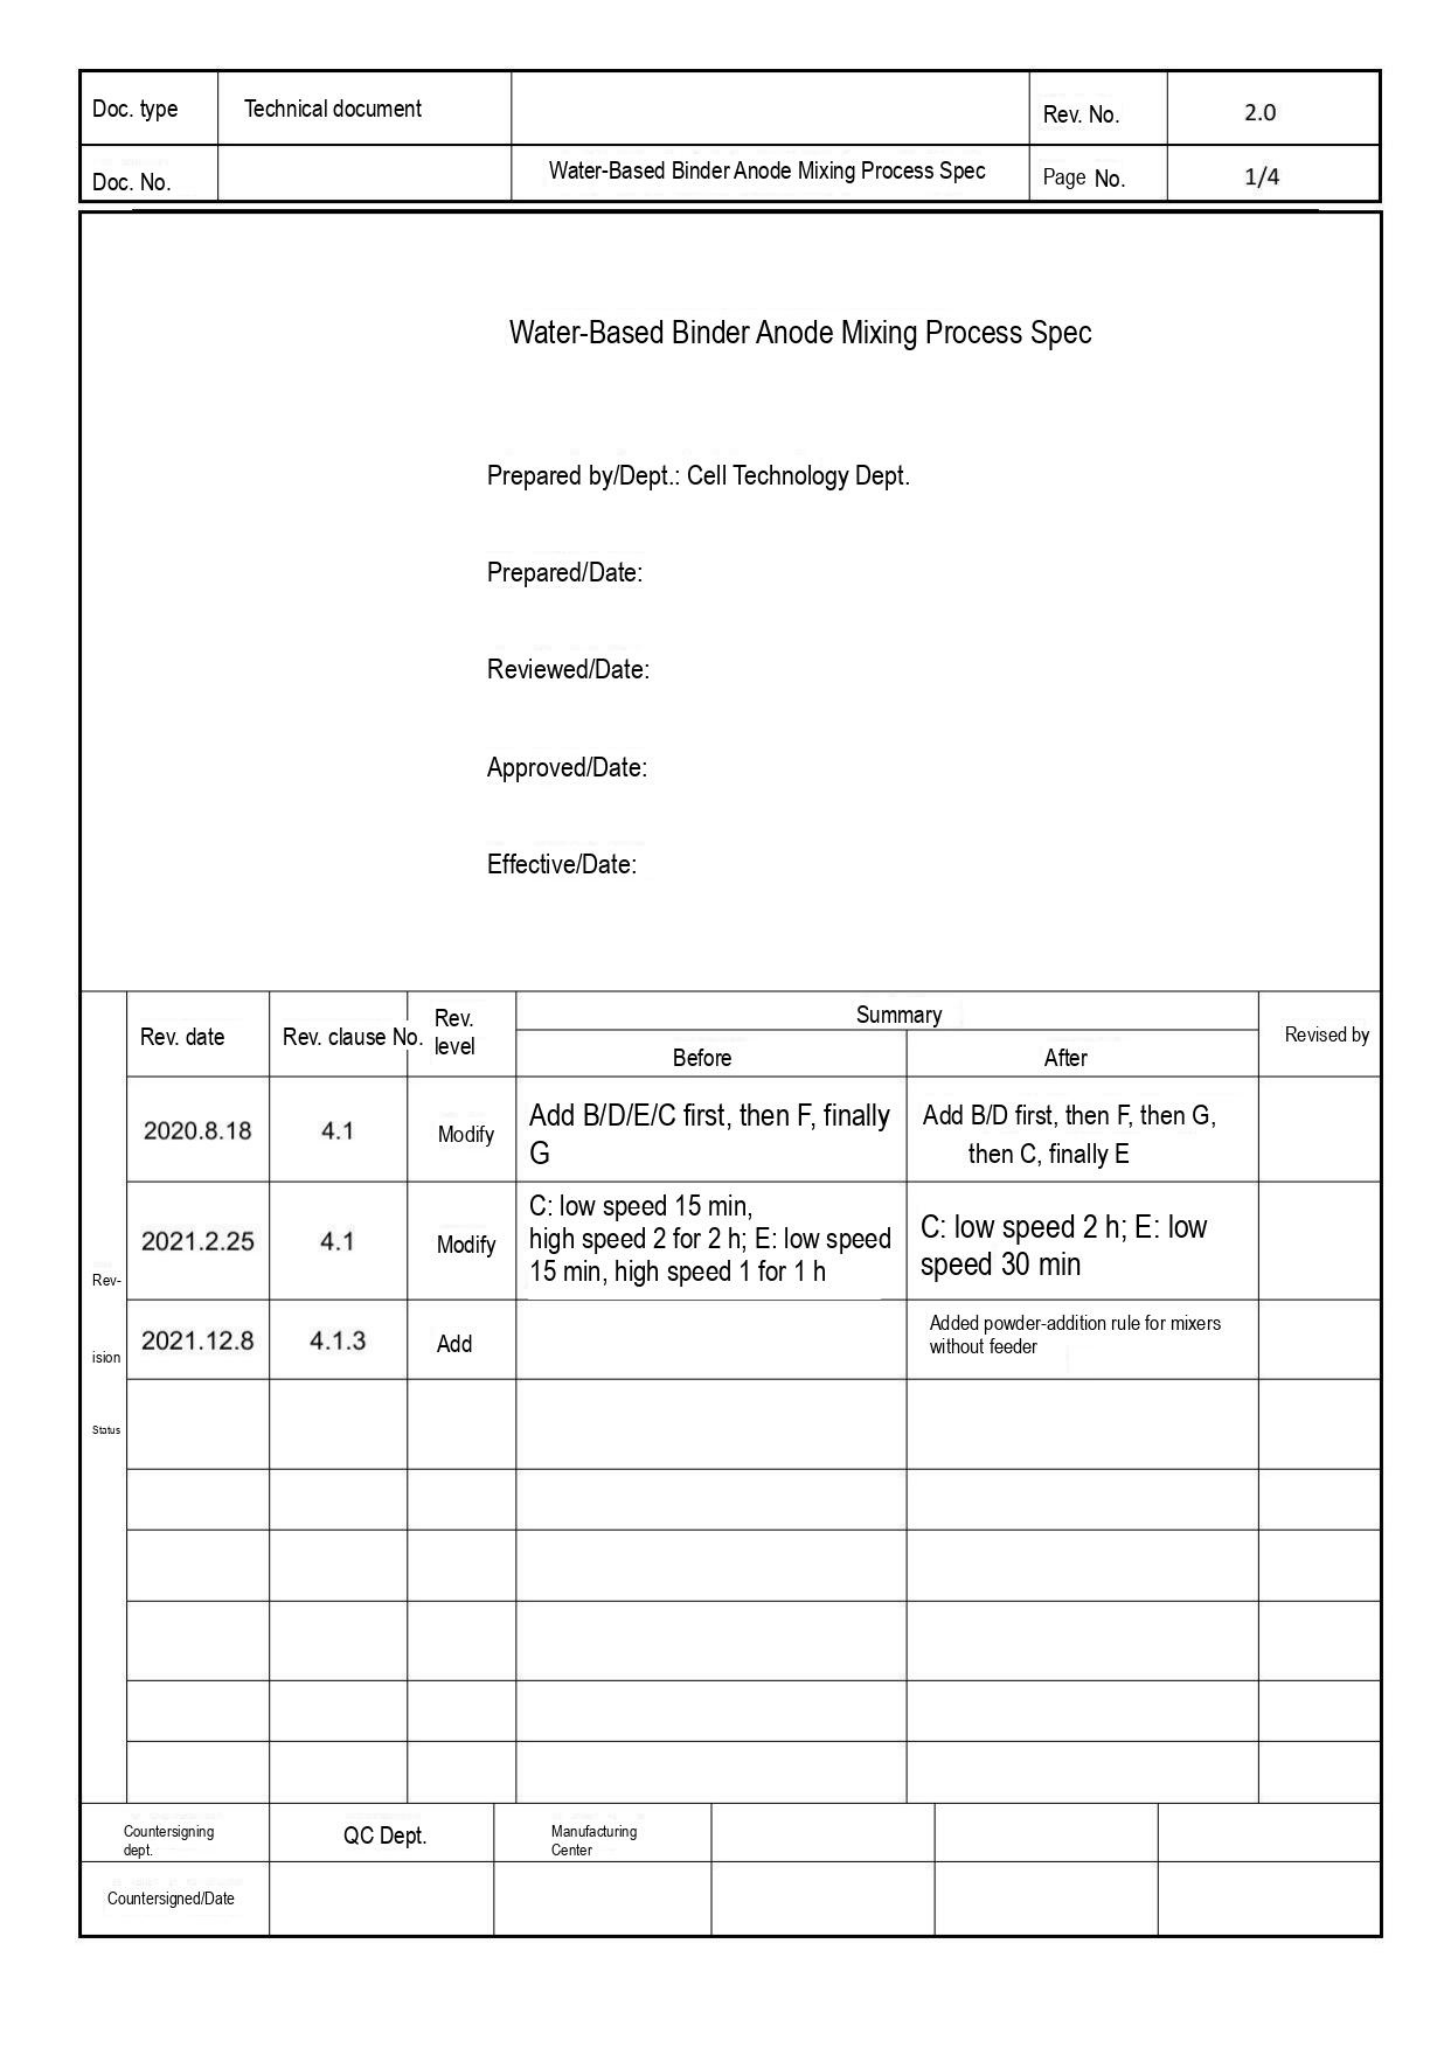| Doc. type | Technical document | | Rev. No. | 2.0 |
|---|---|---|---|---|
| Doc. No. | | Water-Based Binder Anode Mixing Process Spec | Page No. | 1/4 |

Water-Based Binder Anode Mixing Process Spec

Prepared by/Dept.: Cell Technology Dept.

Prepared/Date:

Reviewed/Date:

Approved/Date:

Effective/Date:

| Rev-ision Status | Rev. date | Rev. clause No. | Rev. level | Summary: Before | Summary: After | Revised by |
|---|---|---|---|---|---|---|
| | 2020.8.18 | 4.1 | Modify | Add B/D/E/C first, then F, finally G | Add B/D first, then F, then G, then C, finally E | |
| | 2021.2.25 | 4.1 | Modify | C: low speed 15 min, high speed 2 for 2 h; E: low speed 15 min, high speed 1 for 1 h | C: low speed 2 h; E: low speed 30 min | |
| | 2021.12.8 | 4.1.3 | Add | | Added powder-addition rule for mixers without feeder | |
| | | | | | | |
| | | | | | | |
| | | | | | | |
| | | | | | | |
| | | | | | | |
| | | | | | | |

| Countersigning dept. | QC Dept. | Manufacturing Center | | | |
|---|---|---|---|---|---|
| Countersigned/Date | | | | | |
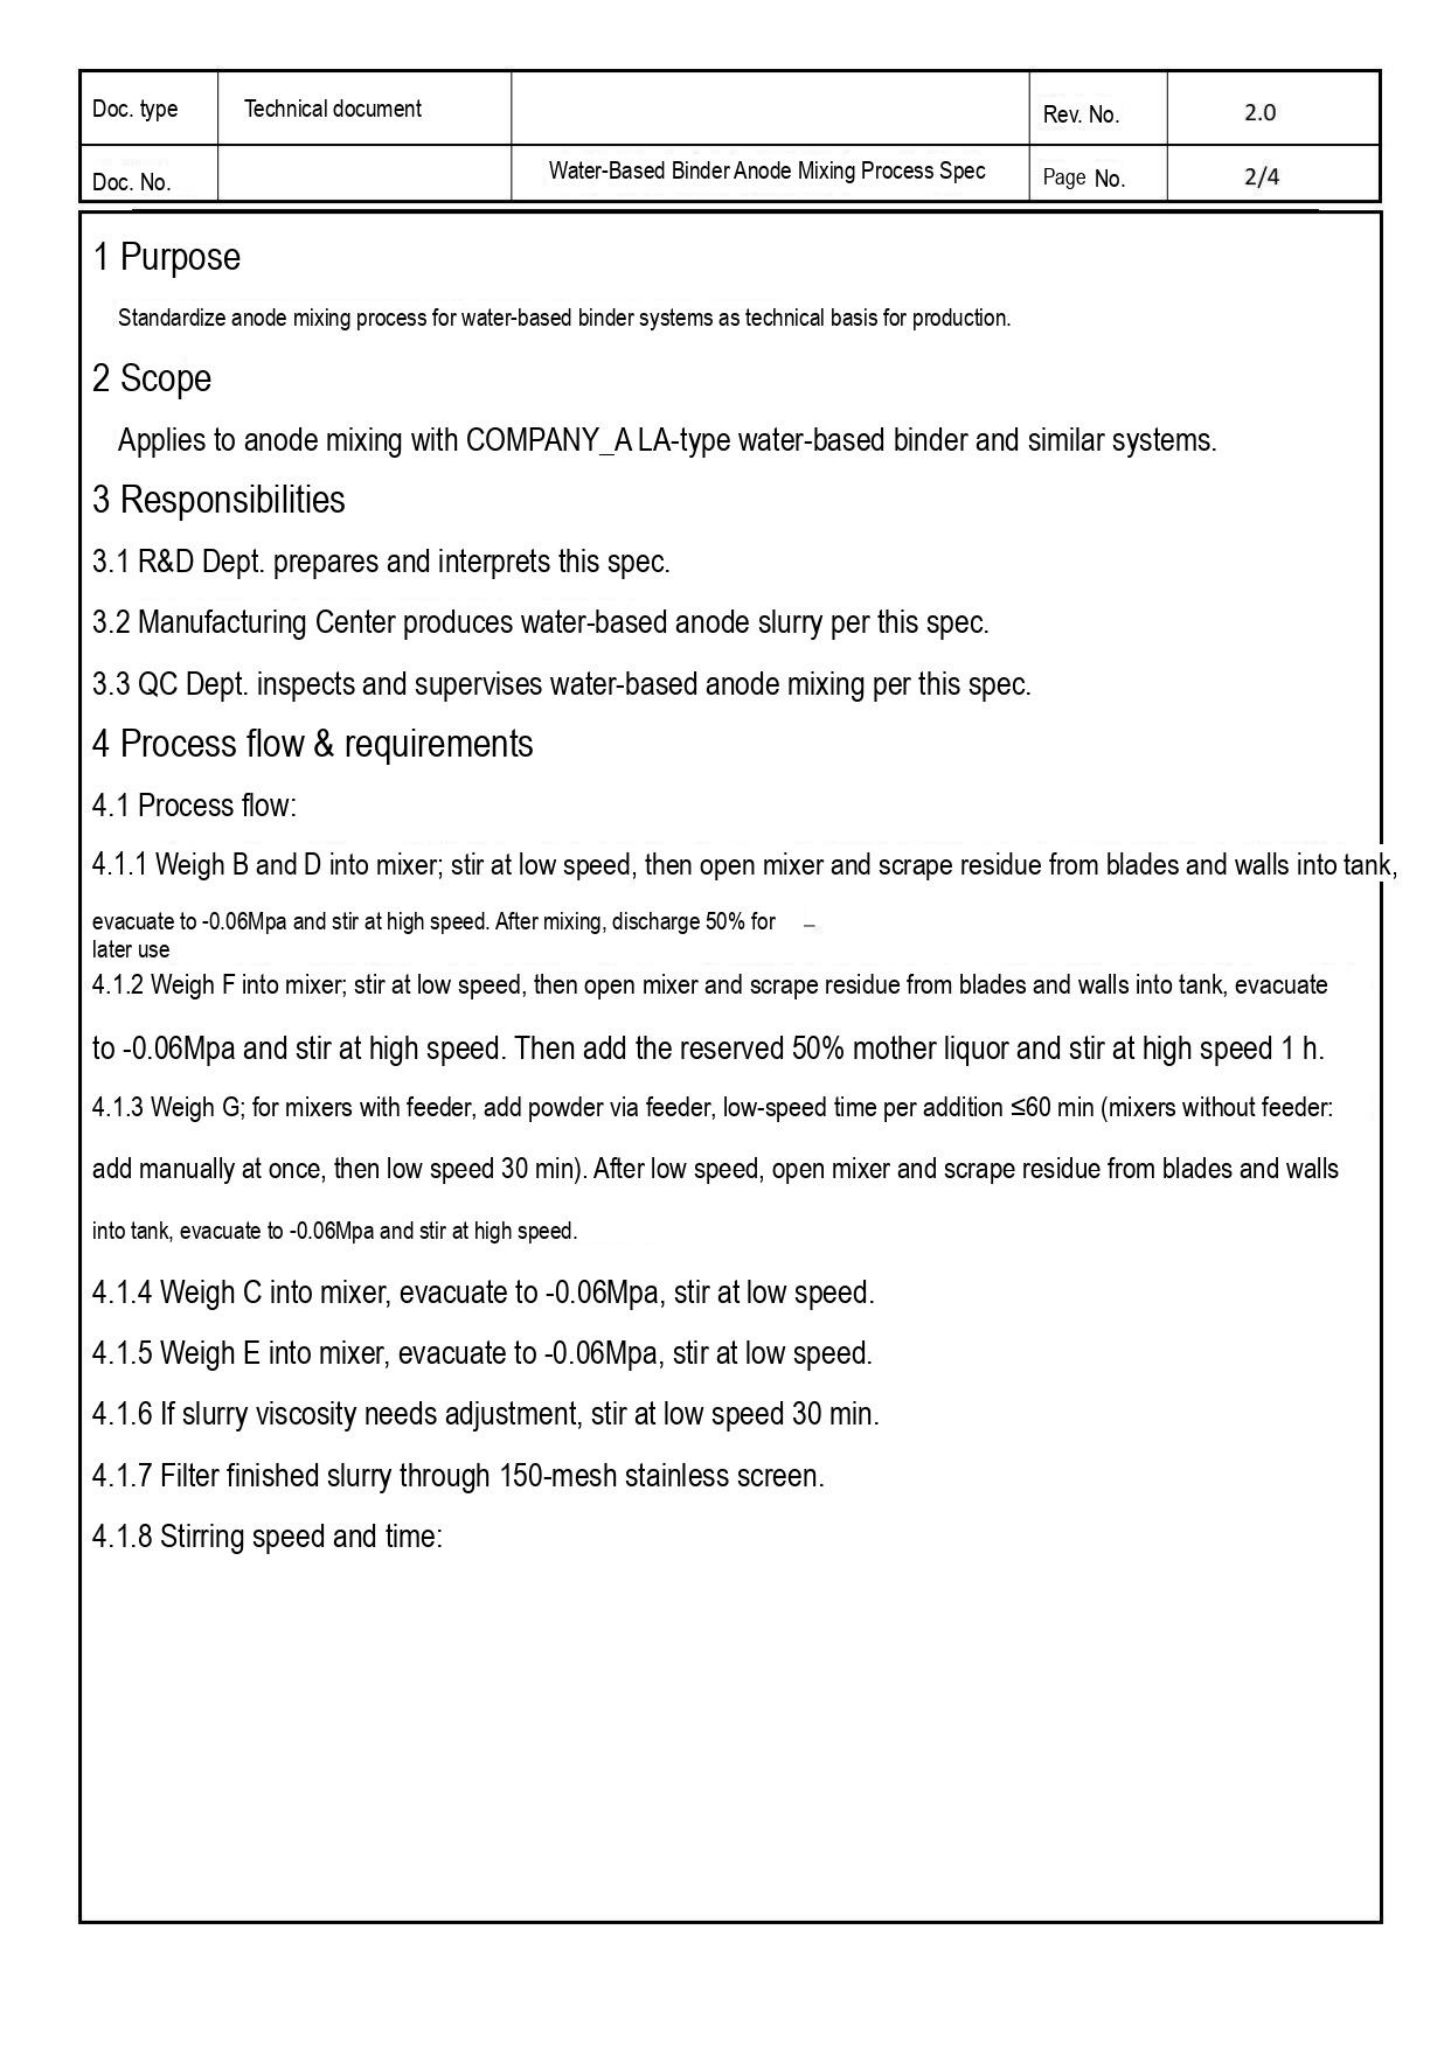| Doc. type | Technical document | | Rev. No. | 2.0 |
|---|---|---|---|---|
| Doc. No. | | Water-Based Binder Anode Mixing Process Spec | Page No. | 2/4 |

1 Purpose

Standardize anode mixing process for water-based binder systems as technical basis for production.

2 Scope

Applies to anode mixing with COMPANY_A LA-type water-based binder and similar systems.

3 Responsibilities

3.1 R&D Dept. prepares and interprets this spec.

3.2 Manufacturing Center produces water-based anode slurry per this spec.

3.3 QC Dept. inspects and supervises water-based anode mixing per this spec.

4 Process flow & requirements

4.1 Process flow:

4.1.1 Weigh B and D into mixer; stir at low speed, then open mixer and scrape residue from blades and walls into tank, evacuate to -0.06Mpa and stir at high speed. After mixing, discharge 50% for later use

4.1.2 Weigh F into mixer; stir at low speed, then open mixer and scrape residue from blades and walls into tank, evacuate to -0.06Mpa and stir at high speed. Then add the reserved 50% mother liquor and stir at high speed 1 h.

4.1.3 Weigh G; for mixers with feeder, add powder via feeder, low-speed time per addition ≤60 min (mixers without feeder: add manually at once, then low speed 30 min). After low speed, open mixer and scrape residue from blades and walls into tank, evacuate to -0.06Mpa and stir at high speed.

4.1.4 Weigh C into mixer, evacuate to -0.06Mpa, stir at low speed.

4.1.5 Weigh E into mixer, evacuate to -0.06Mpa, stir at low speed.

4.1.6 If slurry viscosity needs adjustment, stir at low speed 30 min.

4.1.7 Filter finished slurry through 150-mesh stainless screen.

4.1.8 Stirring speed and time:
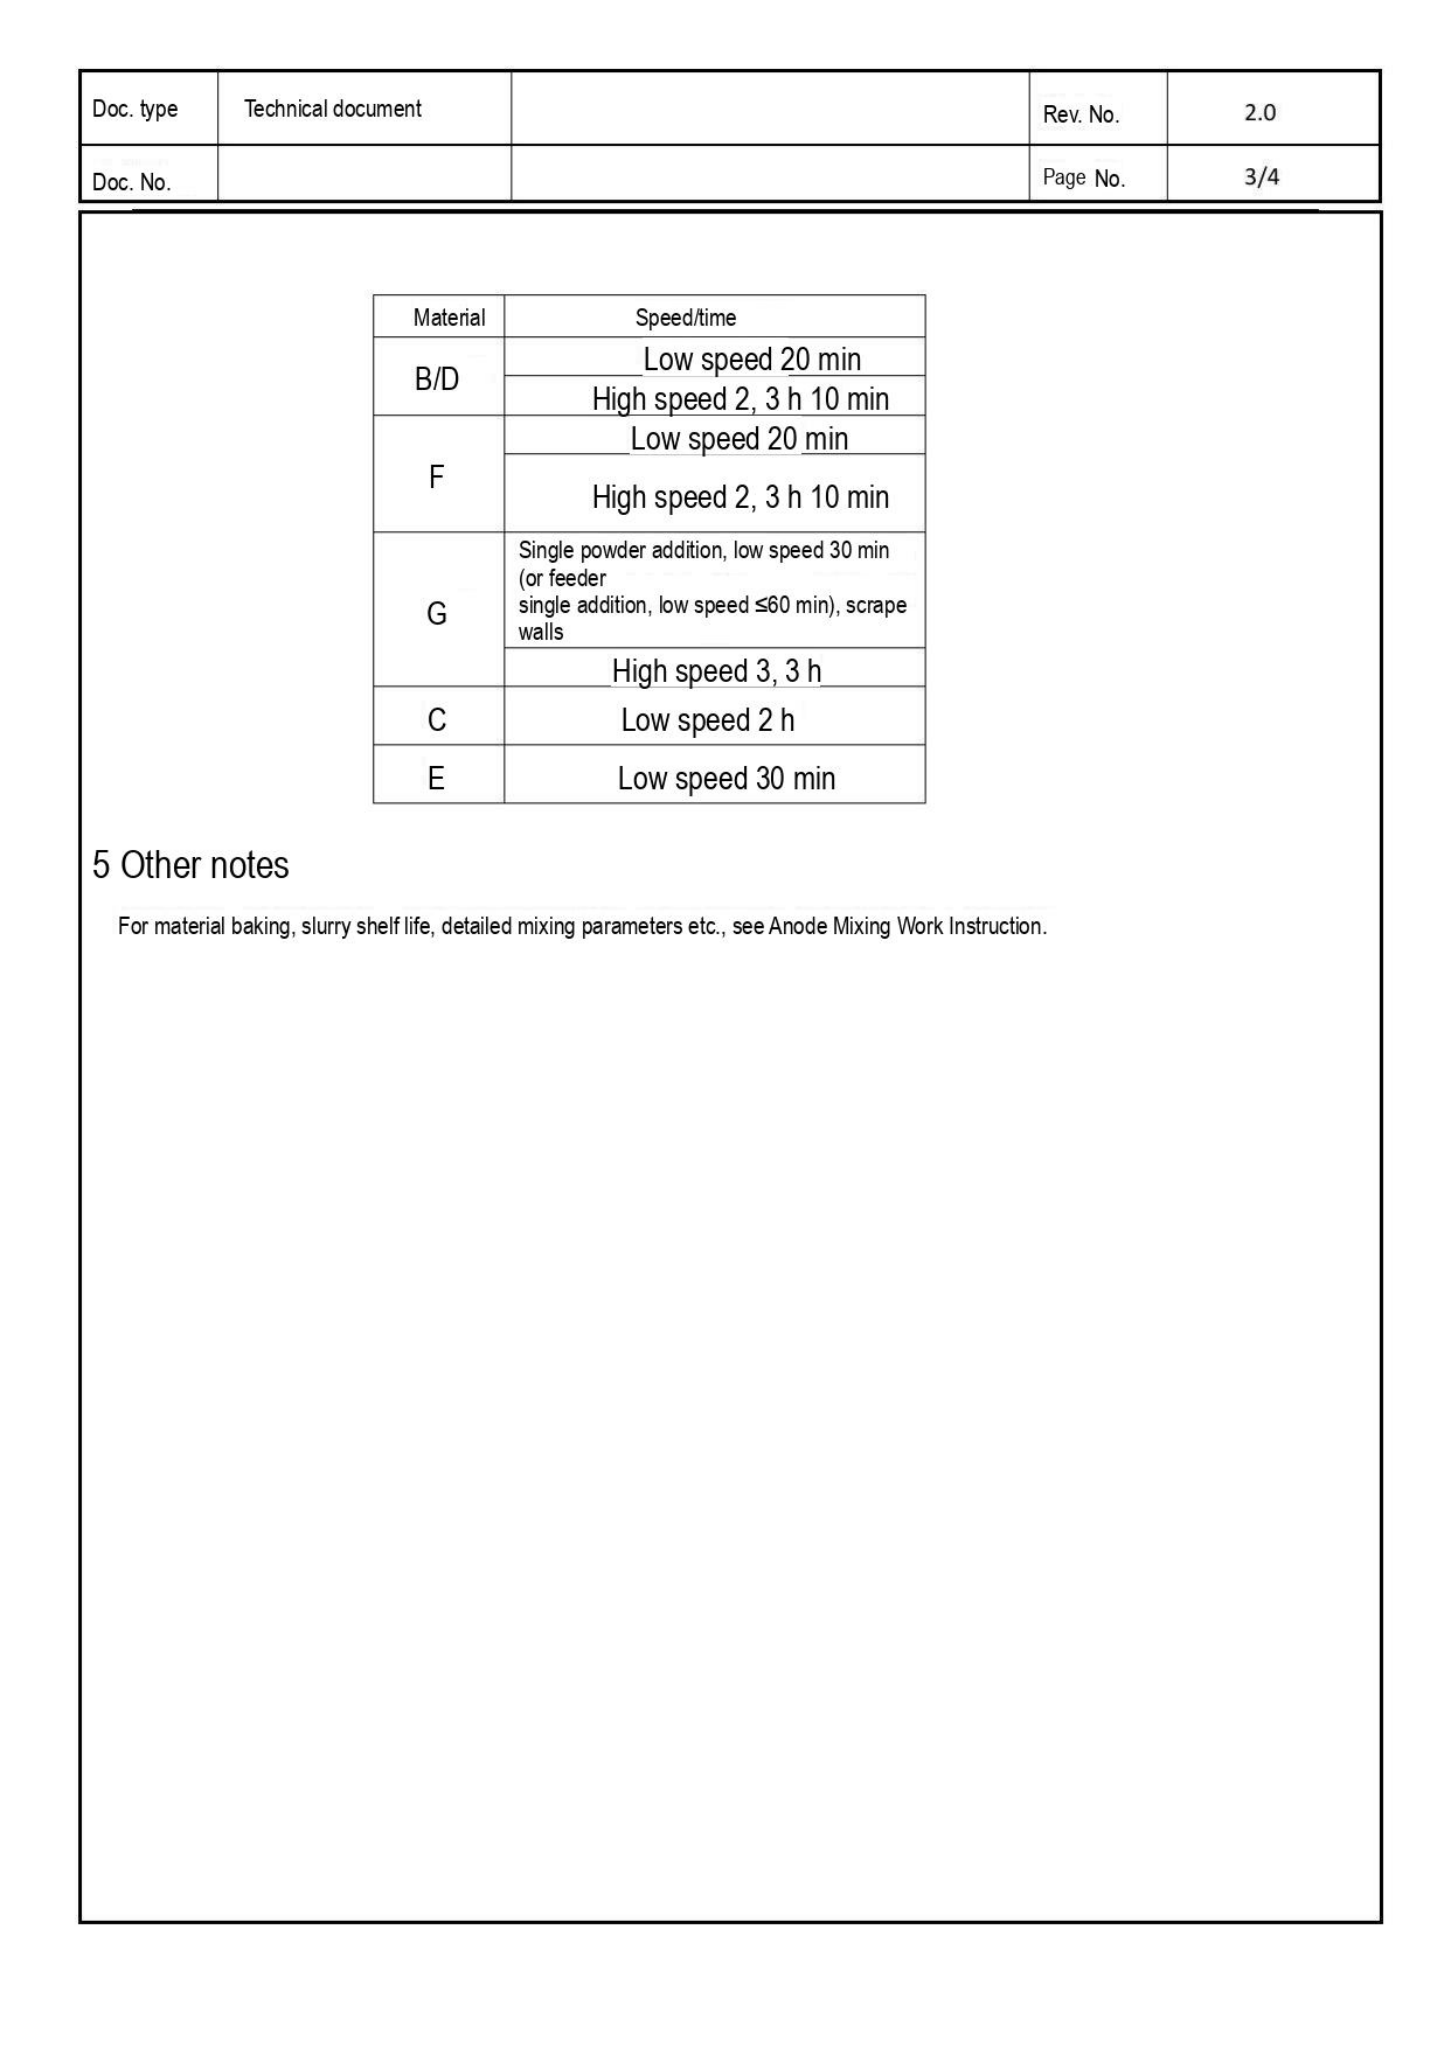| Doc. type | Technical document | | Rev. No. | 2.0 |
|---|---|---|---|---|
| Doc. No. | | | Page No. | 3/4 |

| Material | Speed/time |
|---|---|
| B/D | Low speed 20 min |
| | High speed 2, 3 h 10 min |
| F | Low speed 20 min |
| | High speed 2, 3 h 10 min |
| G | Single powder addition, low speed 30 min (or feeder single addition, low speed ≤60 min), scrape walls |
| | High speed 3, 3 h |
| C | Low speed 2 h |
| E | Low speed 30 min |

5 Other notes

For material baking, slurry shelf life, detailed mixing parameters etc., see Anode Mixing Work Instruction.